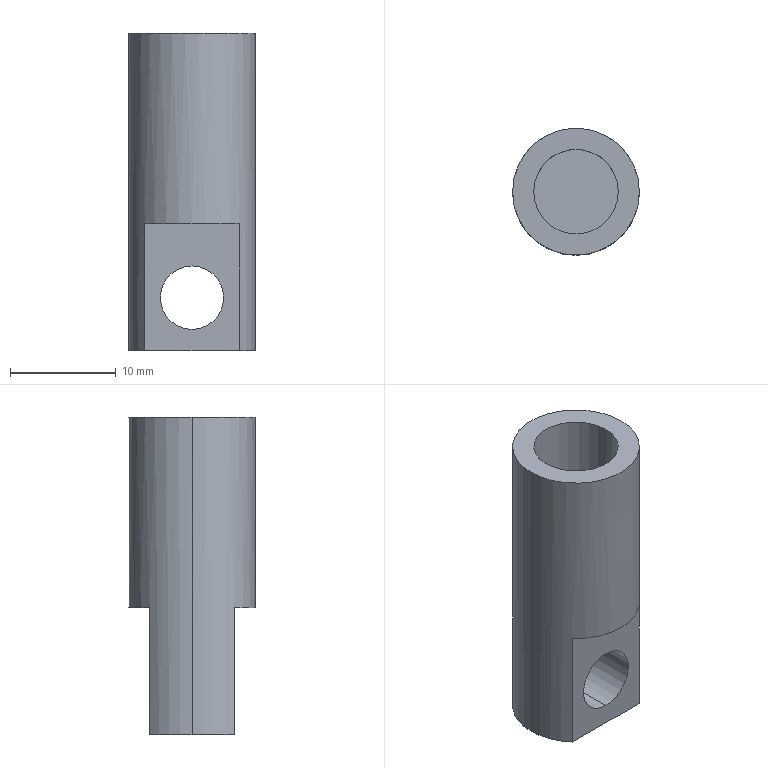Part | SolidWorks | features ICE 3, Extrusion 1, MirrorPattern 1 | 1 solid | 13 faces | box 12 x 12 x 30 mm | volume 2367 mm3 | plane 7 | cylinder 6 | commonest cylinder face diameters 6 x2 8 x2 12 x2
STEP:
#1=CARTESIAN_POINT('',(-4.,0.,20.));
#2=VERTEX_POINT('',#1);
#3=CARTESIAN_POINT('',(4.,0.,20.));
#4=VERTEX_POINT('',#3);
#5=CARTESIAN_POINT('',(0.,0.,20.));
#6=DIRECTION('',(0.,0.,1.));
#7=DIRECTION('',(1.,0.,0.));
#8=AXIS2_PLACEMENT_3D('',#5,#6,#7);
#9=CIRCLE('',#8,4.);
#10=EDGE_CURVE('',#2,#4,#9,.T.);
#11=ORIENTED_EDGE('',*,*,#10,.F.);
#12=CARTESIAN_POINT('',(-4.,0.,30.));
#13=VERTEX_POINT('',#12);
#14=CARTESIAN_POINT('',(-4.,0.,20.));
#15=DIRECTION('',(0.,0.,1.));
#16=VECTOR('',#15,1000.);
#17=LINE('',#14,#16);
#18=EDGE_CURVE('',#2,#13,#17,.T.);
#19=ORIENTED_EDGE('',*,*,#18,.T.);
#20=CARTESIAN_POINT('',(4.,0.,30.));
#21=VERTEX_POINT('',#20);
#22=CARTESIAN_POINT('',(0.,0.,30.));
#23=DIRECTION('',(0.,0.,1.));
#24=DIRECTION('',(1.,0.,0.));
#25=AXIS2_PLACEMENT_3D('',#22,#23,#24);
#26=CIRCLE('',#25,4.);
#27=EDGE_CURVE('',#13,#21,#26,.T.);
#28=ORIENTED_EDGE('',*,*,#27,.T.);
#29=CARTESIAN_POINT('',(4.,0.,20.));
#30=DIRECTION('',(0.,0.,1.));
#31=VECTOR('',#30,1000.);
#32=LINE('',#29,#31);
#33=EDGE_CURVE('',#4,#21,#32,.T.);
#34=ORIENTED_EDGE('',*,*,#33,.F.);
#35=EDGE_LOOP('',(#11,#19,#28,#34));
#36=FACE_OUTER_BOUND('',#35,.T.);
#37=CARTESIAN_POINT('',(0.,0.,20.));
#38=DIRECTION('',(0.,0.,1.));
#39=DIRECTION('',(1.,0.,0.));
#40=AXIS2_PLACEMENT_3D('',#37,#38,#39);
#41=CYLINDRICAL_SURFACE('',#40,4.);
#42=ADVANCED_FACE('',(#36),#41,.F.);
#43=CARTESIAN_POINT('',(0.,4.,8.));
#44=VERTEX_POINT('',#43);
#45=CARTESIAN_POINT('',(0.,4.,2.));
#46=VERTEX_POINT('',#45);
#47=CARTESIAN_POINT('',(0.,4.,5.));
#48=DIRECTION('',(0.,-1.,0.));
#49=DIRECTION('',(0.,0.,-1.));
#50=AXIS2_PLACEMENT_3D('',#47,#48,#49);
#51=CIRCLE('',#50,3.);
#52=EDGE_CURVE('',#44,#46,#51,.T.);
#53=ORIENTED_EDGE('',*,*,#52,.F.);
#54=CARTESIAN_POINT('',(0.,-4.,8.));
#55=VERTEX_POINT('',#54);
#56=CARTESIAN_POINT('',(0.,6.,8.));
#57=DIRECTION('',(0.,-1.,0.));
#58=VECTOR('',#57,1000.);
#59=LINE('',#56,#58);
#60=EDGE_CURVE('',#44,#55,#59,.T.);
#61=ORIENTED_EDGE('',*,*,#60,.T.);
#62=CARTESIAN_POINT('',(0.,-4.,2.));
#63=VERTEX_POINT('',#62);
#64=CARTESIAN_POINT('',(0.,-4.,5.));
#65=DIRECTION('',(0.,1.,0.));
#66=DIRECTION('',(0.,0.,1.));
#67=AXIS2_PLACEMENT_3D('',#64,#65,#66);
#68=CIRCLE('',#67,3.);
#69=EDGE_CURVE('',#63,#55,#68,.T.);
#70=ORIENTED_EDGE('',*,*,#69,.F.);
#71=CARTESIAN_POINT('',(0.,6.,2.));
#72=DIRECTION('',(0.,-1.,0.));
#73=VECTOR('',#72,1000.);
#74=LINE('',#71,#73);
#75=EDGE_CURVE('',#46,#63,#74,.T.);
#76=ORIENTED_EDGE('',*,*,#75,.F.);
#77=EDGE_LOOP('',(#53,#61,#70,#76));
#78=FACE_OUTER_BOUND('',#77,.T.);
#79=CARTESIAN_POINT('',(0.,6.,5.));
#80=DIRECTION('',(0.,-1.,0.));
#81=DIRECTION('',(0.,0.,-1.));
#82=AXIS2_PLACEMENT_3D('',#79,#80,#81);
#83=CYLINDRICAL_SURFACE('',#82,3.);
#84=ADVANCED_FACE('',(#78),#83,.F.);
#85=CARTESIAN_POINT('',(6.,0.,30.));
#86=VERTEX_POINT('',#85);
#87=CARTESIAN_POINT('',(-6.,0.,30.));
#88=VERTEX_POINT('',#87);
#89=CARTESIAN_POINT('',(0.,0.,30.));
#90=DIRECTION('',(0.,0.,1.));
#91=DIRECTION('',(1.,0.,0.));
#92=AXIS2_PLACEMENT_3D('',#89,#90,#91);
#93=CIRCLE('',#92,6.);
#94=EDGE_CURVE('',#86,#88,#93,.T.);
#95=ORIENTED_EDGE('',*,*,#94,.F.);
#96=CARTESIAN_POINT('',(6.,0.,0.));
#97=VERTEX_POINT('',#96);
#98=CARTESIAN_POINT('',(6.,0.,30.));
#99=DIRECTION('',(0.,0.,-1.));
#100=VECTOR('',#99,1000.);
#101=LINE('',#98,#100);
#102=EDGE_CURVE('',#86,#97,#101,.T.);
#103=ORIENTED_EDGE('',*,*,#102,.T.);
#104=CARTESIAN_POINT('',(4.472,4.,0.));
#105=VERTEX_POINT('',#104);
#106=CARTESIAN_POINT('',(0.,0.,0.));
#107=DIRECTION('',(0.,0.,1.));
#108=DIRECTION('',(1.,0.,0.));
#109=AXIS2_PLACEMENT_3D('',#106,#107,#108);
#110=CIRCLE('',#109,6.);
#111=EDGE_CURVE('',#97,#105,#110,.T.);
#112=ORIENTED_EDGE('',*,*,#111,.T.);
#113=CARTESIAN_POINT('',(4.472,4.,12.));
#114=VERTEX_POINT('',#113);
#115=CARTESIAN_POINT('',(4.472,4.,30.));
#116=DIRECTION('',(0.,0.,1.));
#117=VECTOR('',#116,1000.);
#118=LINE('',#115,#117);
#119=EDGE_CURVE('',#105,#114,#118,.T.);
#120=ORIENTED_EDGE('',*,*,#119,.T.);
#121=CARTESIAN_POINT('',(-4.472,4.,12.));
#122=VERTEX_POINT('',#121);
#123=CARTESIAN_POINT('',(0.,0.,12.));
#124=DIRECTION('',(0.,0.,-1.));
#125=DIRECTION('',(-1.,0.,0.));
#126=AXIS2_PLACEMENT_3D('',#123,#124,#125);
#127=CIRCLE('',#126,6.);
#128=EDGE_CURVE('',#122,#114,#127,.T.);
#129=ORIENTED_EDGE('',*,*,#128,.F.);
#130=CARTESIAN_POINT('',(-4.472,4.,0.));
#131=VERTEX_POINT('',#130);
#132=CARTESIAN_POINT('',(-4.472,4.,30.));
#133=DIRECTION('',(0.,0.,-1.));
#134=VECTOR('',#133,1000.);
#135=LINE('',#132,#134);
#136=EDGE_CURVE('',#122,#131,#135,.T.);
#137=ORIENTED_EDGE('',*,*,#136,.T.);
#138=CARTESIAN_POINT('',(-6.,0.,0.));
#139=VERTEX_POINT('',#138);
#140=CARTESIAN_POINT('',(0.,0.,0.));
#141=DIRECTION('',(0.,0.,1.));
#142=DIRECTION('',(1.,0.,0.));
#143=AXIS2_PLACEMENT_3D('',#140,#141,#142);
#144=CIRCLE('',#143,6.);
#145=EDGE_CURVE('',#131,#139,#144,.T.);
#146=ORIENTED_EDGE('',*,*,#145,.T.);
#147=CARTESIAN_POINT('',(-6.,0.,30.));
#148=DIRECTION('',(0.,0.,-1.));
#149=VECTOR('',#148,1000.);
#150=LINE('',#147,#149);
#151=EDGE_CURVE('',#88,#139,#150,.T.);
#152=ORIENTED_EDGE('',*,*,#151,.F.);
#153=EDGE_LOOP('',(#95,#103,#112,#120,#129,#137,#146,#152));
#154=FACE_OUTER_BOUND('',#153,.T.);
#155=CARTESIAN_POINT('',(0.,0.,30.));
#156=DIRECTION('',(0.,0.,-1.));
#157=DIRECTION('',(-1.,0.,0.));
#158=AXIS2_PLACEMENT_3D('',#155,#156,#157);
#159=CYLINDRICAL_SURFACE('',#158,6.);
#160=ADVANCED_FACE('',(#154),#159,.T.);
#161=ORIENTED_EDGE('',*,*,#102,.F.);
#162=CARTESIAN_POINT('',(0.,0.,30.));
#163=DIRECTION('',(0.,0.,1.));
#164=DIRECTION('',(1.,0.,0.));
#165=AXIS2_PLACEMENT_3D('',#162,#163,#164);
#166=CIRCLE('',#165,6.);
#167=EDGE_CURVE('',#88,#86,#166,.T.);
#168=ORIENTED_EDGE('',*,*,#167,.F.);
#169=ORIENTED_EDGE('',*,*,#151,.T.);
#170=CARTESIAN_POINT('',(-4.472,-4.,0.));
#171=VERTEX_POINT('',#170);
#172=CARTESIAN_POINT('',(0.,0.,0.));
#173=DIRECTION('',(0.,0.,1.));
#174=DIRECTION('',(1.,0.,0.));
#175=AXIS2_PLACEMENT_3D('',#172,#173,#174);
#176=CIRCLE('',#175,6.);
#177=EDGE_CURVE('',#139,#171,#176,.T.);
#178=ORIENTED_EDGE('',*,*,#177,.T.);
#179=CARTESIAN_POINT('',(-4.472,-4.,12.));
#180=VERTEX_POINT('',#179);
#181=CARTESIAN_POINT('',(-4.472,-4.,30.));
#182=DIRECTION('',(0.,0.,1.));
#183=VECTOR('',#182,1000.);
#184=LINE('',#181,#183);
#185=EDGE_CURVE('',#171,#180,#184,.T.);
#186=ORIENTED_EDGE('',*,*,#185,.T.);
#187=CARTESIAN_POINT('',(4.472,-4.,12.));
#188=VERTEX_POINT('',#187);
#189=CARTESIAN_POINT('',(0.,0.,12.));
#190=DIRECTION('',(0.,0.,1.));
#191=DIRECTION('',(1.,0.,0.));
#192=AXIS2_PLACEMENT_3D('',#189,#190,#191);
#193=CIRCLE('',#192,6.);
#194=EDGE_CURVE('',#180,#188,#193,.T.);
#195=ORIENTED_EDGE('',*,*,#194,.T.);
#196=CARTESIAN_POINT('',(4.472,-4.,0.));
#197=VERTEX_POINT('',#196);
#198=CARTESIAN_POINT('',(4.472,-4.,30.));
#199=DIRECTION('',(0.,0.,-1.));
#200=VECTOR('',#199,1000.);
#201=LINE('',#198,#200);
#202=EDGE_CURVE('',#188,#197,#201,.T.);
#203=ORIENTED_EDGE('',*,*,#202,.T.);
#204=CARTESIAN_POINT('',(0.,0.,0.));
#205=DIRECTION('',(0.,0.,1.));
#206=DIRECTION('',(1.,0.,0.));
#207=AXIS2_PLACEMENT_3D('',#204,#205,#206);
#208=CIRCLE('',#207,6.);
#209=EDGE_CURVE('',#197,#97,#208,.T.);
#210=ORIENTED_EDGE('',*,*,#209,.T.);
#211=EDGE_LOOP('',(#161,#168,#169,#178,#186,#195,#203,#210));
#212=FACE_OUTER_BOUND('',#211,.T.);
#213=CARTESIAN_POINT('',(0.,0.,30.));
#214=DIRECTION('',(0.,0.,-1.));
#215=DIRECTION('',(-1.,0.,0.));
#216=AXIS2_PLACEMENT_3D('',#213,#214,#215);
#217=CYLINDRICAL_SURFACE('',#216,6.);
#218=ADVANCED_FACE('',(#212),#217,.T.);
#219=CARTESIAN_POINT('',(0.,0.,30.));
#220=DIRECTION('',(0.,0.,1.));
#221=DIRECTION('',(1.,0.,0.));
#222=AXIS2_PLACEMENT_3D('',#219,#220,#221);
#223=CIRCLE('',#222,4.);
#224=EDGE_CURVE('',#21,#13,#223,.T.);
#225=ORIENTED_EDGE('',*,*,#224,.F.);
#226=ORIENTED_EDGE('',*,*,#27,.F.);
#227=EDGE_LOOP('',(#225,#226));
#228=FACE_BOUND('',#227,.T.);
#229=ORIENTED_EDGE('',*,*,#167,.T.);
#230=ORIENTED_EDGE('',*,*,#94,.T.);
#231=EDGE_LOOP('',(#229,#230));
#232=FACE_OUTER_BOUND('',#231,.T.);
#233=CARTESIAN_POINT('',(0.,0.,30.));
#234=DIRECTION('',(0.,0.,1.));
#235=DIRECTION('',(1.,0.,0.));
#236=AXIS2_PLACEMENT_3D('',#233,#234,#235);
#237=PLANE('',#236);
#238=ADVANCED_FACE('',(#228,#232),#237,.T.);
#239=ORIENTED_EDGE('',*,*,#145,.F.);
#240=CARTESIAN_POINT('',(0.,4.,0.));
#241=DIRECTION('',(1.,0.,0.));
#242=VECTOR('',#241,1000.);
#243=LINE('',#240,#242);
#244=EDGE_CURVE('',#131,#105,#243,.T.);
#245=ORIENTED_EDGE('',*,*,#244,.T.);
#246=ORIENTED_EDGE('',*,*,#111,.F.);
#247=ORIENTED_EDGE('',*,*,#209,.F.);
#248=CARTESIAN_POINT('',(0.,-4.,0.));
#249=DIRECTION('',(-1.,0.,0.));
#250=VECTOR('',#249,1000.);
#251=LINE('',#248,#250);
#252=EDGE_CURVE('',#197,#171,#251,.T.);
#253=ORIENTED_EDGE('',*,*,#252,.T.);
#254=ORIENTED_EDGE('',*,*,#177,.F.);
#255=EDGE_LOOP('',(#239,#245,#246,#247,#253,#254));
#256=FACE_OUTER_BOUND('',#255,.T.);
#257=CARTESIAN_POINT('',(0.,0.,0.));
#258=DIRECTION('',(0.,0.,1.));
#259=DIRECTION('',(1.,0.,0.));
#260=AXIS2_PLACEMENT_3D('',#257,#258,#259);
#261=PLANE('',#260);
#262=ADVANCED_FACE('',(#256),#261,.F.);
#263=CARTESIAN_POINT('',(-10.88,-4.,12.));
#264=DIRECTION('',(1.,0.,0.));
#265=VECTOR('',#264,1000.);
#266=LINE('',#263,#265);
#267=EDGE_CURVE('',#180,#188,#266,.T.);
#268=ORIENTED_EDGE('',*,*,#267,.T.);
#269=ORIENTED_EDGE('',*,*,#194,.F.);
#270=EDGE_LOOP('',(#268,#269));
#271=FACE_OUTER_BOUND('',#270,.T.);
#272=CARTESIAN_POINT('',(-10.88,-14.,12.));
#273=DIRECTION('',(0.,0.,1.));
#274=DIRECTION('',(1.,0.,0.));
#275=AXIS2_PLACEMENT_3D('',#272,#273,#274);
#276=PLANE('',#275);
#277=ADVANCED_FACE('',(#271),#276,.F.);
#278=ORIENTED_EDGE('',*,*,#69,.T.);
#279=CARTESIAN_POINT('',(0.,-4.,5.));
#280=DIRECTION('',(0.,1.,0.));
#281=DIRECTION('',(0.,0.,1.));
#282=AXIS2_PLACEMENT_3D('',#279,#280,#281);
#283=CIRCLE('',#282,3.);
#284=EDGE_CURVE('',#55,#63,#283,.T.);
#285=ORIENTED_EDGE('',*,*,#284,.T.);
#286=EDGE_LOOP('',(#278,#285));
#287=FACE_BOUND('',#286,.T.);
#288=ORIENTED_EDGE('',*,*,#267,.F.);
#289=ORIENTED_EDGE('',*,*,#185,.F.);
#290=ORIENTED_EDGE('',*,*,#252,.F.);
#291=ORIENTED_EDGE('',*,*,#202,.F.);
#292=EDGE_LOOP('',(#288,#289,#290,#291));
#293=FACE_OUTER_BOUND('',#292,.T.);
#294=CARTESIAN_POINT('',(0.,-4.,0.));
#295=DIRECTION('',(0.,1.,0.));
#296=DIRECTION('',(0.,0.,1.));
#297=AXIS2_PLACEMENT_3D('',#294,#295,#296);
#298=PLANE('',#297);
#299=ADVANCED_FACE('',(#287,#293),#298,.F.);
#300=ORIENTED_EDGE('',*,*,#128,.T.);
#301=CARTESIAN_POINT('',(-10.88,4.,12.));
#302=DIRECTION('',(1.,0.,0.));
#303=VECTOR('',#302,1000.);
#304=LINE('',#301,#303);
#305=EDGE_CURVE('',#122,#114,#304,.T.);
#306=ORIENTED_EDGE('',*,*,#305,.F.);
#307=EDGE_LOOP('',(#300,#306));
#308=FACE_OUTER_BOUND('',#307,.T.);
#309=CARTESIAN_POINT('',(-10.88,14.,12.));
#310=DIRECTION('',(0.,0.,-1.));
#311=DIRECTION('',(-1.,0.,0.));
#312=AXIS2_PLACEMENT_3D('',#309,#310,#311);
#313=PLANE('',#312);
#314=ADVANCED_FACE('',(#308),#313,.T.);
#315=CARTESIAN_POINT('',(0.,4.,5.));
#316=DIRECTION('',(0.,-1.,0.));
#317=DIRECTION('',(0.,0.,-1.));
#318=AXIS2_PLACEMENT_3D('',#315,#316,#317);
#319=CIRCLE('',#318,3.);
#320=EDGE_CURVE('',#46,#44,#319,.T.);
#321=ORIENTED_EDGE('',*,*,#320,.T.);
#322=ORIENTED_EDGE('',*,*,#52,.T.);
#323=EDGE_LOOP('',(#321,#322));
#324=FACE_BOUND('',#323,.T.);
#325=ORIENTED_EDGE('',*,*,#305,.T.);
#326=ORIENTED_EDGE('',*,*,#119,.F.);
#327=ORIENTED_EDGE('',*,*,#244,.F.);
#328=ORIENTED_EDGE('',*,*,#136,.F.);
#329=EDGE_LOOP('',(#325,#326,#327,#328));
#330=FACE_OUTER_BOUND('',#329,.T.);
#331=CARTESIAN_POINT('',(0.,4.,0.));
#332=DIRECTION('',(0.,-1.,0.));
#333=DIRECTION('',(0.,0.,1.));
#334=AXIS2_PLACEMENT_3D('',#331,#332,#333);
#335=PLANE('',#334);
#336=ADVANCED_FACE('',(#324,#330),#335,.F.);
#337=ORIENTED_EDGE('',*,*,#60,.F.);
#338=ORIENTED_EDGE('',*,*,#320,.F.);
#339=ORIENTED_EDGE('',*,*,#75,.T.);
#340=ORIENTED_EDGE('',*,*,#284,.F.);
#341=EDGE_LOOP('',(#337,#338,#339,#340));
#342=FACE_OUTER_BOUND('',#341,.T.);
#343=CARTESIAN_POINT('',(0.,6.,5.));
#344=DIRECTION('',(0.,-1.,0.));
#345=DIRECTION('',(0.,0.,-1.));
#346=AXIS2_PLACEMENT_3D('',#343,#344,#345);
#347=CYLINDRICAL_SURFACE('',#346,3.);
#348=ADVANCED_FACE('',(#342),#347,.F.);
#349=ORIENTED_EDGE('',*,*,#18,.F.);
#350=CARTESIAN_POINT('',(0.,0.,20.));
#351=DIRECTION('',(0.,0.,1.));
#352=DIRECTION('',(1.,0.,0.));
#353=AXIS2_PLACEMENT_3D('',#350,#351,#352);
#354=CIRCLE('',#353,4.);
#355=EDGE_CURVE('',#4,#2,#354,.T.);
#356=ORIENTED_EDGE('',*,*,#355,.F.);
#357=ORIENTED_EDGE('',*,*,#33,.T.);
#358=ORIENTED_EDGE('',*,*,#224,.T.);
#359=EDGE_LOOP('',(#349,#356,#357,#358));
#360=FACE_OUTER_BOUND('',#359,.T.);
#361=CARTESIAN_POINT('',(0.,0.,20.));
#362=DIRECTION('',(0.,0.,1.));
#363=DIRECTION('',(1.,0.,0.));
#364=AXIS2_PLACEMENT_3D('',#361,#362,#363);
#365=CYLINDRICAL_SURFACE('',#364,4.);
#366=ADVANCED_FACE('',(#360),#365,.F.);
#367=ORIENTED_EDGE('',*,*,#355,.T.);
#368=ORIENTED_EDGE('',*,*,#10,.T.);
#369=EDGE_LOOP('',(#367,#368));
#370=FACE_OUTER_BOUND('',#369,.T.);
#371=CARTESIAN_POINT('',(0.,0.,20.));
#372=DIRECTION('',(0.,0.,1.));
#373=DIRECTION('',(1.,0.,0.));
#374=AXIS2_PLACEMENT_3D('',#371,#372,#373);
#375=PLANE('',#374);
#376=ADVANCED_FACE('',(#370),#375,.T.);
#377=CLOSED_SHELL('',(#42,#84,#160,#218,#238,#262,#277,#299,#314,#336,#348,#366,#376));
#378=MANIFOLD_SOLID_BREP('',#377);
#379=CARTESIAN_POINT('',(0.,0.,0.));
#380=DIRECTION('',(0.,0.,1.));
#381=DIRECTION('',(1.,0.,0.));
#382=AXIS2_PLACEMENT_3D('',#379,#380,#381);
#383=(LENGTH_UNIT()NAMED_UNIT(*)SI_UNIT(.MILLI.,.METRE.));
#384=UNCERTAINTY_MEASURE_WITH_UNIT(LENGTH_MEASURE(0.00001),#383,'','');
#385=(NAMED_UNIT(*)PLANE_ANGLE_UNIT()SI_UNIT($,.RADIAN.));
#386=(NAMED_UNIT(*)SI_UNIT($,.STERADIAN.)SOLID_ANGLE_UNIT());
#387=(GEOMETRIC_REPRESENTATION_CONTEXT(3)GLOBAL_UNCERTAINTY_ASSIGNED_CONTEXT((#384))GLOBAL_UNIT_ASSIGNED_CONTEXT((#383,#385,#386))REPRESENTATION_CONTEXT('',''));
#388=ADVANCED_BREP_SHAPE_REPRESENTATION('',(#378,#382),#387);